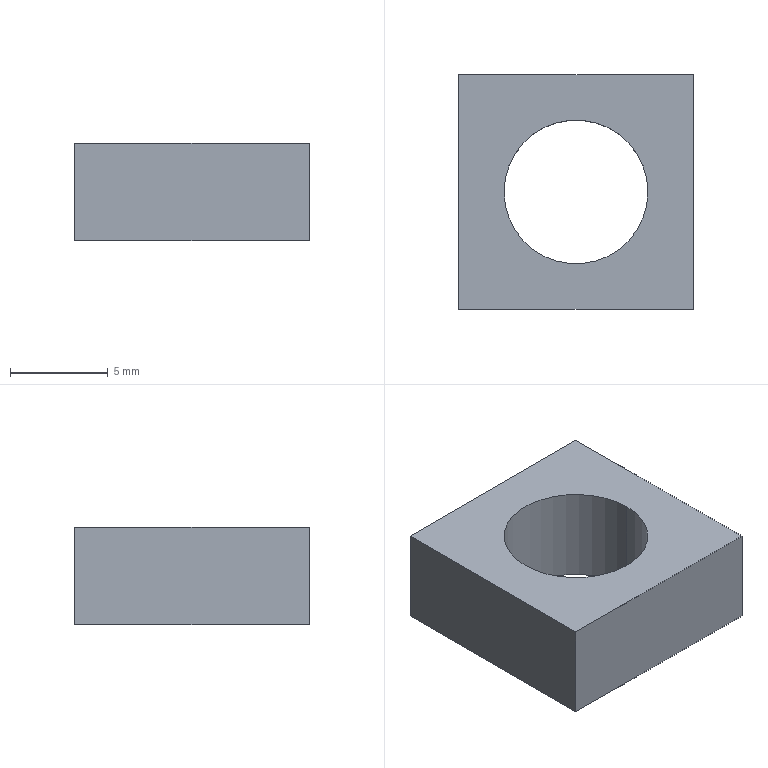Part | SolidWorks | features Extrusion 1 | 1 solid | 8 faces | box 12 x 12 x 5 mm | volume 507.902 mm3 | plane 6 | cylinder 2 | commonest cylinder face diameters 7.349 x2
STEP:
#1=CARTESIAN_POINT('',(-30.74,0.,-5.));
#2=VERTEX_POINT('',#1);
#3=CARTESIAN_POINT('',(-23.391,0.,-5.));
#4=VERTEX_POINT('',#3);
#5=CARTESIAN_POINT('',(-27.066,0.,-5.));
#6=DIRECTION('',(0.,0.,1.));
#7=DIRECTION('',(1.,0.,0.));
#8=AXIS2_PLACEMENT_3D('',#5,#6,#7);
#9=CIRCLE('',#8,3.675);
#10=EDGE_CURVE('',#2,#4,#9,.T.);
#11=ORIENTED_EDGE('',*,*,#10,.F.);
#12=CARTESIAN_POINT('',(-30.74,0.,0.));
#13=VERTEX_POINT('',#12);
#14=CARTESIAN_POINT('',(-30.74,0.,-5.));
#15=DIRECTION('',(0.,0.,1.));
#16=VECTOR('',#15,1000.);
#17=LINE('',#14,#16);
#18=EDGE_CURVE('',#2,#13,#17,.T.);
#19=ORIENTED_EDGE('',*,*,#18,.T.);
#20=CARTESIAN_POINT('',(-23.391,0.,0.));
#21=VERTEX_POINT('',#20);
#22=CARTESIAN_POINT('',(-27.066,0.,0.));
#23=DIRECTION('',(0.,0.,1.));
#24=DIRECTION('',(1.,0.,0.));
#25=AXIS2_PLACEMENT_3D('',#22,#23,#24);
#26=CIRCLE('',#25,3.675);
#27=EDGE_CURVE('',#13,#21,#26,.T.);
#28=ORIENTED_EDGE('',*,*,#27,.T.);
#29=CARTESIAN_POINT('',(-23.391,0.,-5.));
#30=DIRECTION('',(0.,0.,1.));
#31=VECTOR('',#30,1000.);
#32=LINE('',#29,#31);
#33=EDGE_CURVE('',#4,#21,#32,.T.);
#34=ORIENTED_EDGE('',*,*,#33,.F.);
#35=EDGE_LOOP('',(#11,#19,#28,#34));
#36=FACE_OUTER_BOUND('',#35,.T.);
#37=CARTESIAN_POINT('',(-27.066,0.,-5.));
#38=DIRECTION('',(0.,0.,1.));
#39=DIRECTION('',(1.,0.,0.));
#40=AXIS2_PLACEMENT_3D('',#37,#38,#39);
#41=CYLINDRICAL_SURFACE('',#40,3.675);
#42=ADVANCED_FACE('',(#36),#41,.F.);
#43=CARTESIAN_POINT('',(-21.066,-6.,0.));
#44=VERTEX_POINT('',#43);
#45=CARTESIAN_POINT('',(-21.066,6.,0.));
#46=VERTEX_POINT('',#45);
#47=CARTESIAN_POINT('',(-21.066,6.,0.));
#48=DIRECTION('',(0.,1.,0.));
#49=VECTOR('',#48,1000.);
#50=LINE('',#47,#49);
#51=EDGE_CURVE('',#44,#46,#50,.T.);
#52=ORIENTED_EDGE('',*,*,#51,.F.);
#53=CARTESIAN_POINT('',(-21.066,-6.,-5.));
#54=VERTEX_POINT('',#53);
#55=CARTESIAN_POINT('',(-21.066,-6.,-5.));
#56=DIRECTION('',(0.,0.,1.));
#57=VECTOR('',#56,1000.);
#58=LINE('',#55,#57);
#59=EDGE_CURVE('',#54,#44,#58,.T.);
#60=ORIENTED_EDGE('',*,*,#59,.F.);
#61=CARTESIAN_POINT('',(-21.066,6.,-5.));
#62=VERTEX_POINT('',#61);
#63=CARTESIAN_POINT('',(-21.066,6.,-5.));
#64=DIRECTION('',(0.,1.,0.));
#65=VECTOR('',#64,1000.);
#66=LINE('',#63,#65);
#67=EDGE_CURVE('',#54,#62,#66,.T.);
#68=ORIENTED_EDGE('',*,*,#67,.T.);
#69=CARTESIAN_POINT('',(-21.066,6.,-5.));
#70=DIRECTION('',(0.,0.,1.));
#71=VECTOR('',#70,1000.);
#72=LINE('',#69,#71);
#73=EDGE_CURVE('',#62,#46,#72,.T.);
#74=ORIENTED_EDGE('',*,*,#73,.T.);
#75=EDGE_LOOP('',(#52,#60,#68,#74));
#76=FACE_OUTER_BOUND('',#75,.T.);
#77=CARTESIAN_POINT('',(-21.066,6.,-5.));
#78=DIRECTION('',(1.,0.,0.));
#79=DIRECTION('',(0.,1.,0.));
#80=AXIS2_PLACEMENT_3D('',#77,#78,#79);
#81=PLANE('',#80);
#82=ADVANCED_FACE('',(#76),#81,.T.);
#83=CARTESIAN_POINT('',(-33.066,-6.,0.));
#84=VERTEX_POINT('',#83);
#85=CARTESIAN_POINT('',(-33.066,-6.,0.));
#86=DIRECTION('',(1.,0.,0.));
#87=VECTOR('',#86,1000.);
#88=LINE('',#85,#87);
#89=EDGE_CURVE('',#84,#44,#88,.T.);
#90=ORIENTED_EDGE('',*,*,#89,.F.);
#91=CARTESIAN_POINT('',(-33.066,-6.,-5.));
#92=VERTEX_POINT('',#91);
#93=CARTESIAN_POINT('',(-33.066,-6.,-5.));
#94=DIRECTION('',(0.,0.,1.));
#95=VECTOR('',#94,1000.);
#96=LINE('',#93,#95);
#97=EDGE_CURVE('',#92,#84,#96,.T.);
#98=ORIENTED_EDGE('',*,*,#97,.F.);
#99=CARTESIAN_POINT('',(-33.066,-6.,-5.));
#100=DIRECTION('',(1.,0.,0.));
#101=VECTOR('',#100,1000.);
#102=LINE('',#99,#101);
#103=EDGE_CURVE('',#92,#54,#102,.T.);
#104=ORIENTED_EDGE('',*,*,#103,.T.);
#105=ORIENTED_EDGE('',*,*,#59,.T.);
#106=EDGE_LOOP('',(#90,#98,#104,#105));
#107=FACE_OUTER_BOUND('',#106,.T.);
#108=CARTESIAN_POINT('',(-33.066,-6.,-5.));
#109=DIRECTION('',(0.,-1.,0.));
#110=DIRECTION('',(0.,0.,-1.));
#111=AXIS2_PLACEMENT_3D('',#108,#109,#110);
#112=PLANE('',#111);
#113=ADVANCED_FACE('',(#107),#112,.T.);
#114=CARTESIAN_POINT('',(-33.066,6.,0.));
#115=VERTEX_POINT('',#114);
#116=CARTESIAN_POINT('',(-33.066,6.,0.));
#117=DIRECTION('',(0.,-1.,0.));
#118=VECTOR('',#117,1000.);
#119=LINE('',#116,#118);
#120=EDGE_CURVE('',#115,#84,#119,.T.);
#121=ORIENTED_EDGE('',*,*,#120,.F.);
#122=CARTESIAN_POINT('',(-33.066,6.,-5.));
#123=VERTEX_POINT('',#122);
#124=CARTESIAN_POINT('',(-33.066,6.,-5.));
#125=DIRECTION('',(0.,0.,1.));
#126=VECTOR('',#125,1000.);
#127=LINE('',#124,#126);
#128=EDGE_CURVE('',#123,#115,#127,.T.);
#129=ORIENTED_EDGE('',*,*,#128,.F.);
#130=CARTESIAN_POINT('',(-33.066,6.,-5.));
#131=DIRECTION('',(0.,-1.,0.));
#132=VECTOR('',#131,1000.);
#133=LINE('',#130,#132);
#134=EDGE_CURVE('',#123,#92,#133,.T.);
#135=ORIENTED_EDGE('',*,*,#134,.T.);
#136=ORIENTED_EDGE('',*,*,#97,.T.);
#137=EDGE_LOOP('',(#121,#129,#135,#136));
#138=FACE_OUTER_BOUND('',#137,.T.);
#139=CARTESIAN_POINT('',(-33.066,6.,-5.));
#140=DIRECTION('',(-1.,0.,0.));
#141=DIRECTION('',(0.,0.,1.));
#142=AXIS2_PLACEMENT_3D('',#139,#140,#141);
#143=PLANE('',#142);
#144=ADVANCED_FACE('',(#138),#143,.T.);
#145=CARTESIAN_POINT('',(-33.066,6.,0.));
#146=DIRECTION('',(-1.,0.,0.));
#147=VECTOR('',#146,1000.);
#148=LINE('',#145,#147);
#149=EDGE_CURVE('',#46,#115,#148,.T.);
#150=ORIENTED_EDGE('',*,*,#149,.F.);
#151=ORIENTED_EDGE('',*,*,#73,.F.);
#152=CARTESIAN_POINT('',(-33.066,6.,-5.));
#153=DIRECTION('',(-1.,0.,0.));
#154=VECTOR('',#153,1000.);
#155=LINE('',#152,#154);
#156=EDGE_CURVE('',#62,#123,#155,.T.);
#157=ORIENTED_EDGE('',*,*,#156,.T.);
#158=ORIENTED_EDGE('',*,*,#128,.T.);
#159=EDGE_LOOP('',(#150,#151,#157,#158));
#160=FACE_OUTER_BOUND('',#159,.T.);
#161=CARTESIAN_POINT('',(-33.066,6.,-5.));
#162=DIRECTION('',(0.,1.,0.));
#163=DIRECTION('',(0.,0.,1.));
#164=AXIS2_PLACEMENT_3D('',#161,#162,#163);
#165=PLANE('',#164);
#166=ADVANCED_FACE('',(#160),#165,.T.);
#167=CARTESIAN_POINT('',(-27.066,0.,-5.));
#168=DIRECTION('',(0.,0.,1.));
#169=DIRECTION('',(1.,0.,0.));
#170=AXIS2_PLACEMENT_3D('',#167,#168,#169);
#171=CIRCLE('',#170,3.675);
#172=EDGE_CURVE('',#4,#2,#171,.T.);
#173=ORIENTED_EDGE('',*,*,#172,.T.);
#174=ORIENTED_EDGE('',*,*,#10,.T.);
#175=EDGE_LOOP('',(#173,#174));
#176=FACE_BOUND('',#175,.T.);
#177=ORIENTED_EDGE('',*,*,#67,.F.);
#178=ORIENTED_EDGE('',*,*,#103,.F.);
#179=ORIENTED_EDGE('',*,*,#134,.F.);
#180=ORIENTED_EDGE('',*,*,#156,.F.);
#181=EDGE_LOOP('',(#177,#178,#179,#180));
#182=FACE_OUTER_BOUND('',#181,.T.);
#183=CARTESIAN_POINT('',(0.,0.,-5.));
#184=DIRECTION('',(0.,0.,1.));
#185=DIRECTION('',(1.,0.,0.));
#186=AXIS2_PLACEMENT_3D('',#183,#184,#185);
#187=PLANE('',#186);
#188=ADVANCED_FACE('',(#176,#182),#187,.F.);
#189=CARTESIAN_POINT('',(-27.066,0.,0.));
#190=DIRECTION('',(0.,0.,1.));
#191=DIRECTION('',(1.,0.,0.));
#192=AXIS2_PLACEMENT_3D('',#189,#190,#191);
#193=CIRCLE('',#192,3.675);
#194=EDGE_CURVE('',#21,#13,#193,.T.);
#195=ORIENTED_EDGE('',*,*,#194,.F.);
#196=ORIENTED_EDGE('',*,*,#27,.F.);
#197=EDGE_LOOP('',(#195,#196));
#198=FACE_BOUND('',#197,.T.);
#199=ORIENTED_EDGE('',*,*,#51,.T.);
#200=ORIENTED_EDGE('',*,*,#149,.T.);
#201=ORIENTED_EDGE('',*,*,#120,.T.);
#202=ORIENTED_EDGE('',*,*,#89,.T.);
#203=EDGE_LOOP('',(#199,#200,#201,#202));
#204=FACE_OUTER_BOUND('',#203,.T.);
#205=CARTESIAN_POINT('',(0.,0.,0.));
#206=DIRECTION('',(0.,0.,1.));
#207=DIRECTION('',(1.,0.,0.));
#208=AXIS2_PLACEMENT_3D('',#205,#206,#207);
#209=PLANE('',#208);
#210=ADVANCED_FACE('',(#198,#204),#209,.T.);
#211=ORIENTED_EDGE('',*,*,#18,.F.);
#212=ORIENTED_EDGE('',*,*,#172,.F.);
#213=ORIENTED_EDGE('',*,*,#33,.T.);
#214=ORIENTED_EDGE('',*,*,#194,.T.);
#215=EDGE_LOOP('',(#211,#212,#213,#214));
#216=FACE_OUTER_BOUND('',#215,.T.);
#217=CARTESIAN_POINT('',(-27.066,0.,-5.));
#218=DIRECTION('',(0.,0.,1.));
#219=DIRECTION('',(1.,0.,0.));
#220=AXIS2_PLACEMENT_3D('',#217,#218,#219);
#221=CYLINDRICAL_SURFACE('',#220,3.675);
#222=ADVANCED_FACE('',(#216),#221,.F.);
#223=CLOSED_SHELL('',(#42,#82,#113,#144,#166,#188,#210,#222));
#224=MANIFOLD_SOLID_BREP('',#223);
#225=CARTESIAN_POINT('',(0.,0.,0.));
#226=DIRECTION('',(0.,0.,1.));
#227=DIRECTION('',(1.,0.,0.));
#228=AXIS2_PLACEMENT_3D('',#225,#226,#227);
#229=(LENGTH_UNIT()NAMED_UNIT(*)SI_UNIT(.MILLI.,.METRE.));
#230=UNCERTAINTY_MEASURE_WITH_UNIT(LENGTH_MEASURE(0.00001),#229,'','');
#231=(NAMED_UNIT(*)PLANE_ANGLE_UNIT()SI_UNIT($,.RADIAN.));
#232=(NAMED_UNIT(*)SI_UNIT($,.STERADIAN.)SOLID_ANGLE_UNIT());
#233=(GEOMETRIC_REPRESENTATION_CONTEXT(3)GLOBAL_UNCERTAINTY_ASSIGNED_CONTEXT((#230))GLOBAL_UNIT_ASSIGNED_CONTEXT((#229,#231,#232))REPRESENTATION_CONTEXT('',''));
#234=ADVANCED_BREP_SHAPE_REPRESENTATION('',(#224,#228),#233);